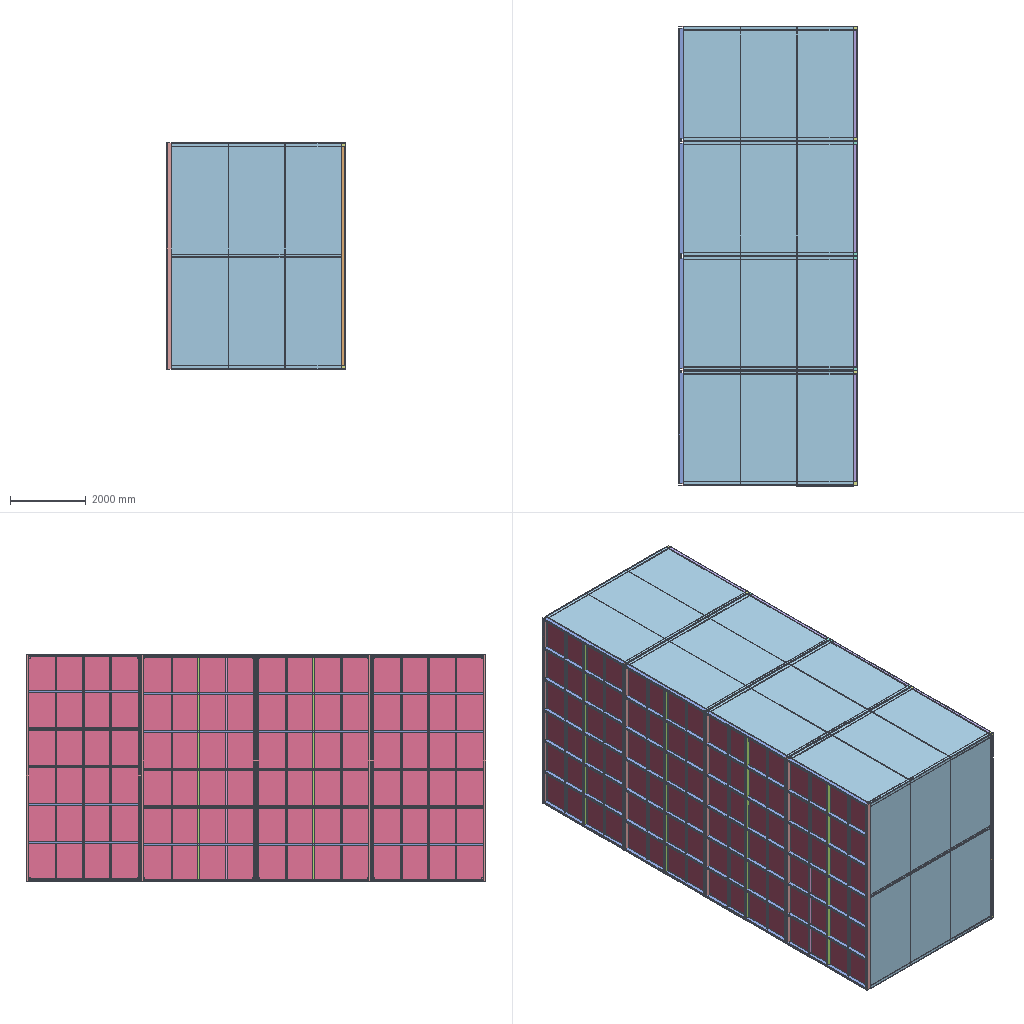Assembly | SolidWorks | 15 different items | 142 placed | box 4720 x 12172 x 6011 mm
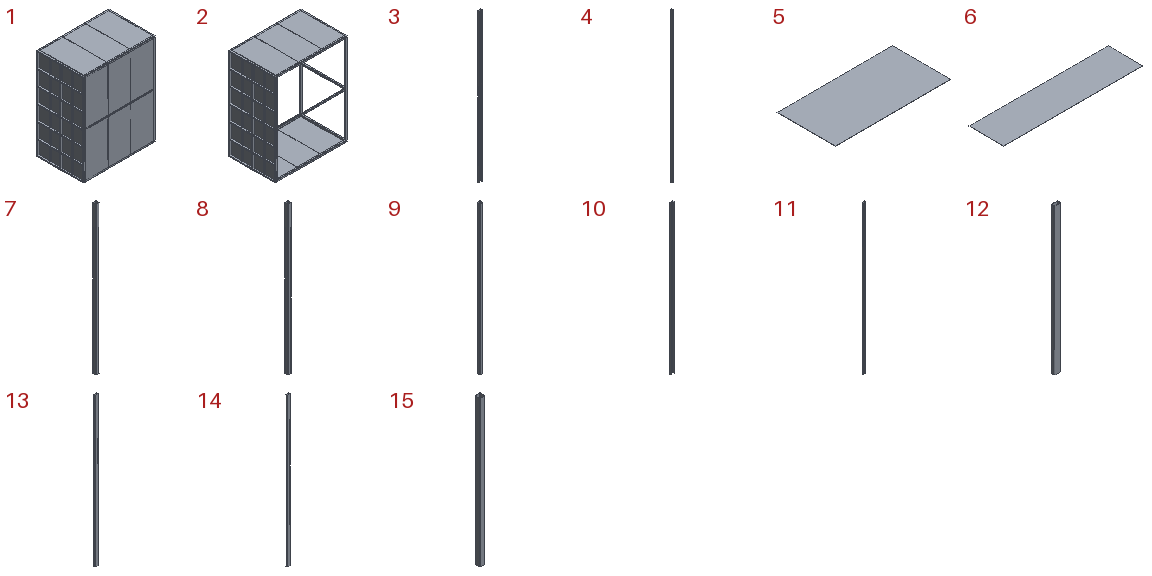Parts list (item | name | quantity | parent item | size | volume | features):
1 | (subassembly) | x2 | - | 4720 x 3046 x 6011 mm | 585161679 mm3 | features ReferencePattern 20, LocalLPattern 7, LayoutProfileFeature 1
2 | (subassembly) | x2 | - | 4720 x 3040 x 6011 mm | 422081679 mm3 | features ReferencePattern 15, LocalLPattern 6, LayoutProfileFeature 1
3 | - | x1 | - | 120 x 50 x 6000 mm | 8487812 mm3 | features Extrusion 1
4 | - | x8 | in 1, 2 | 40 x 60 x 5880 mm | 2698361 mm3 | features Extrusion 1
5 | - | x36 | in 1, 2 | 3000 x 1510 x 6 mm | 27180000 mm3 | features Extrusion 1
6 | - | x8 | in 1, 2 | 6000 x 1510 x 6 mm | 54360000 mm3 | features Extrusion 1
7 | - | x8 | in 2 | 100 x 100 x 4600 mm | 8443849 mm3 | features Extrusion 1
8 | - | x8 | in 1 | 100 x 100 x 4600 mm | 8443849 mm3 | features Extrusion 1
9 | - | x8 | in 1, 2 | 100 x 100 x 5800 mm | 10646593 mm3 | features Extrusion 1
10 | - | x8 | in 1, 2 | 100 x 50 x 4500 mm | 5749980 mm3 | features Extrusion 1
11 | - | x1 | - | 100 x 50 x 6000 mm | 7666640 mm3 | features Extrusion 1
12 | - | x28 | in 1, 2 | 120 x 60 x 2920 mm | 4776009 mm3 | features Extrusion 1
13 | - | x4 | in 1, 2 | 120 x 60 x 5880 mm | 9617442 mm3 | features Extrusion 1
14 | - | x8 | in 1, 2 | 120 x 60 x 6000 mm | 9813717 mm3 | features Extrusion 1
15 | - | x12 | in 1, 2 | 100 x 100 x 2840 mm | 5213159 mm3 | features Extrusion 1
Mates (type | each side: item.copy, entity, surface, feature):
In the top assembly
Coincident | 12.1 face plane Boss-Extrude1 | 12.2 face plane Boss-Extrude1
Coincident | 14.1 face plane Boss-Extrude1 | 7.1 face plane Boss-Extrude1
Coincident | 14.1 face plane Boss-Extrude1 | 14.2 face plane Boss-Extrude1
Coincident | 5.1 face plane Boss-Extrude1 | 5.2 face plane Boss-Extrude1
Coincident | 9.1 face plane Boss-Extrude1 | 9.2 face plane Boss-Extrude1 | 2 times
Coincident | 5.3 face plane Boss-Extrude1 | 5.4 face plane Boss-Extrude1
Coincident | 9.3 face plane Boss-Extrude1 | 15.1 face plane Boss-Extrude1
Coincident | 7.2 face plane Boss-Extrude1 | 8.1 face plane Boss-Extrude1
In subassembly 1
Coincident | 14.3 face plane Boss-Extrude1 | 12.3 face plane Boss-Extrude1 | 3 times
Coincident | 12.3 face plane Boss-Extrude1 | 14.4 face plane Boss-Extrude1 | 3 times
Coincident | 14.4 face plane Boss-Extrude1 | 12.4 face plane Boss-Extrude1 | 3 times
Coincident | 12.3 face plane Boss-Extrude1 | 13.1 face plane Boss-Extrude1 | 2 times
DistanceDim | 14.4 face plane Boss-Extrude1 | 13.1 face plane Boss-Extrude1
Coincident | 12.4 face plane Boss-Extrude1 | 4.1 face plane Boss-Extrude1 | 2 times
DistanceDim | 4.1 face plane Boss-Extrude1 | 13.1 face plane Boss-Extrude1
Coincident | 14.3 face plane Boss-Extrude1 | 8.2 face plane Boss-Extrude1 | 2 times
Coincident | 12.3 face plane Boss-Extrude1 | 8.2 face plane Boss-Extrude1
Coincident | 8.2 face plane Boss-Extrude1 | 9.4 face plane Boss-Extrude1 | 3 times
Coincident | 8.3 face plane Boss-Extrude1 | 9.5 face plane Boss-Extrude1 | 3 times
Coincident | 8.3 face plane Boss-Extrude1 | 15.2 face plane Boss-Extrude1 | 3 times
Coincident | 8.4 face plane Boss-Extrude1 | 15.3 face plane Boss-Extrude1 | 3 times
Coincident | 9.4 face plane Boss-Extrude1 | 10.1 face plane Boss-Extrude1 | 2 times
DistanceDim | 10.1 face plane Boss-Extrude1 | 8.4 face plane Boss-Extrude1
Coincident | 14.4 face plane Boss-Extrude1 | 10.2 face plane Boss-Extrude1 | 2 times
Coincident | 10.1 face plane Boss-Extrude1 | 10.2 face plane Boss-Extrude1
Coincident | 14.4 face plane Boss-Extrude1 | 6.1 face plane Boss-Extrude1 | 2 times
Coincident | 12.3 face plane Boss-Extrude1 | 6.1 face plane Boss-Extrude1
Coincident | 14.3 face plane Boss-Extrude1 | 6.2 face plane Boss-Extrude1 | 2 times
Coincident | 12.4 face plane Boss-Extrude1 | 6.2 face plane Boss-Extrude1
Coincident | 8.5 face plane Boss-Extrude1 | 5.5 face plane Boss-Extrude1
Coincident | 6.2 face plane Boss-Extrude1 | 5.5 face plane Boss-Extrude1
DistanceDim | 8.4 face plane Boss-Extrude1 | 5.5 face plane Boss-Extrude1
Coincident | 14.4 face plane Boss-Extrude1 | 5.6 face plane Boss-Extrude1
Coincident | 8.5 face plane Boss-Extrude1 | 5.6 face plane Boss-Extrude1
Coincident | 5.5 face plane Boss-Extrude1 | 5.6 face plane Boss-Extrude1
In subassembly 2
Coincident | 14.3 face plane Boss-Extrude1 | 12.3 face plane Boss-Extrude1 | 3 times
Coincident | 12.3 face plane Boss-Extrude1 | 14.4 face plane Boss-Extrude1 | 3 times
Coincident | 14.4 face plane Boss-Extrude1 | 12.4 face plane Boss-Extrude1 | 3 times
Coincident | 12.3 face plane Boss-Extrude1 | 13.1 face plane Boss-Extrude1 | 2 times
DistanceDim | 14.4 face plane Boss-Extrude1 | 13.1 face plane Boss-Extrude1
Coincident | 12.4 face plane Boss-Extrude1 | 4.1 face plane Boss-Extrude1 | 2 times
DistanceDim | 4.1 face plane Boss-Extrude1 | 13.1 face plane Boss-Extrude1
Coincident | 14.3 face plane Boss-Extrude1 | 7.3 face plane Boss-Extrude1 | 2 times
Coincident | 12.3 face plane Boss-Extrude1 | 7.3 face plane Boss-Extrude1
Coincident | 7.3 face plane Boss-Extrude1 | 9.4 face plane Boss-Extrude1 | 3 times
Coincident | 7.4 face plane Boss-Extrude1 | 9.5 face plane Boss-Extrude1 | 3 times
Coincident | 7.4 face plane Boss-Extrude1 | 15.2 face plane Boss-Extrude1 | 3 times
Coincident | 7.5 face plane Boss-Extrude1 | 15.3 face plane Boss-Extrude1 | 3 times
Coincident | 9.4 face plane Boss-Extrude1 | 10.1 face plane Boss-Extrude1 | 2 times
DistanceDim | 10.1 face plane Boss-Extrude1 | 7.5 face plane Boss-Extrude1
Coincident | 14.4 face plane Boss-Extrude1 | 10.2 face plane Boss-Extrude1 | 2 times
Coincident | 10.1 face plane Boss-Extrude1 | 10.2 face plane Boss-Extrude1
Coincident | 14.4 face plane Boss-Extrude1 | 6.1 face plane Boss-Extrude1 | 2 times
Coincident | 12.3 face plane Boss-Extrude1 | 6.1 face plane Boss-Extrude1
Coincident | 14.3 face plane Boss-Extrude1 | 6.2 face plane Boss-Extrude1 | 2 times
Coincident | 12.4 face plane Boss-Extrude1 | 6.2 face plane Boss-Extrude1
Coincident | 7.6 face plane Boss-Extrude1 | 5.5 face plane Boss-Extrude1
Coincident | 6.2 face plane Boss-Extrude1 | 5.5 face plane Boss-Extrude1
DistanceDim | 7.5 face plane Boss-Extrude1 | 5.5 face plane Boss-Extrude1